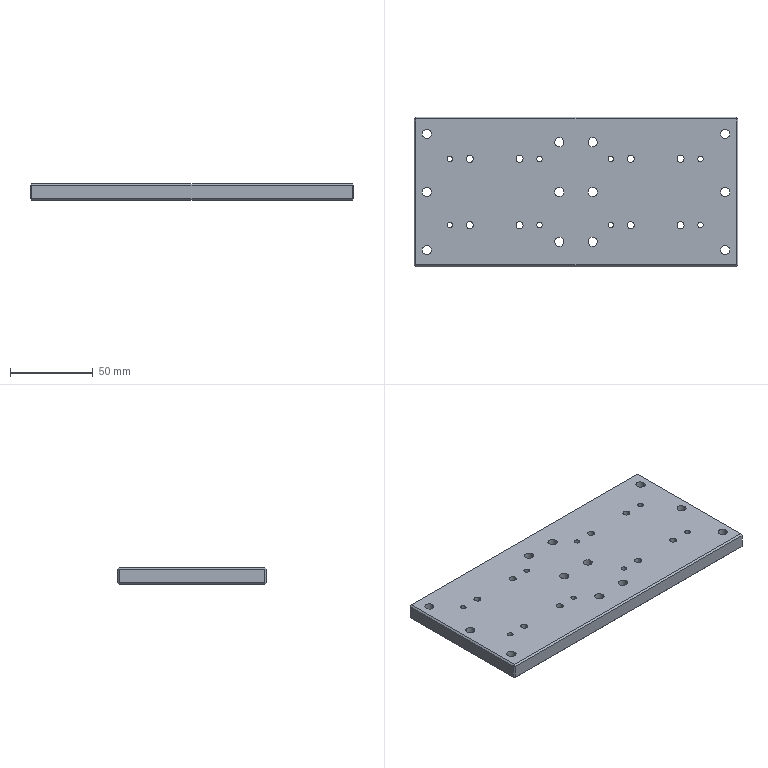Part | STEP file | 07-04 camera mounting plate | 1 solid | 118 faces | box 195 x 90 x 10 mm | volume 166722 mm3 | cylinder 80 | plane 38 | commonest cylinder face diameters 5.5 x24 10 x24 3.3 x16 4.2 x16